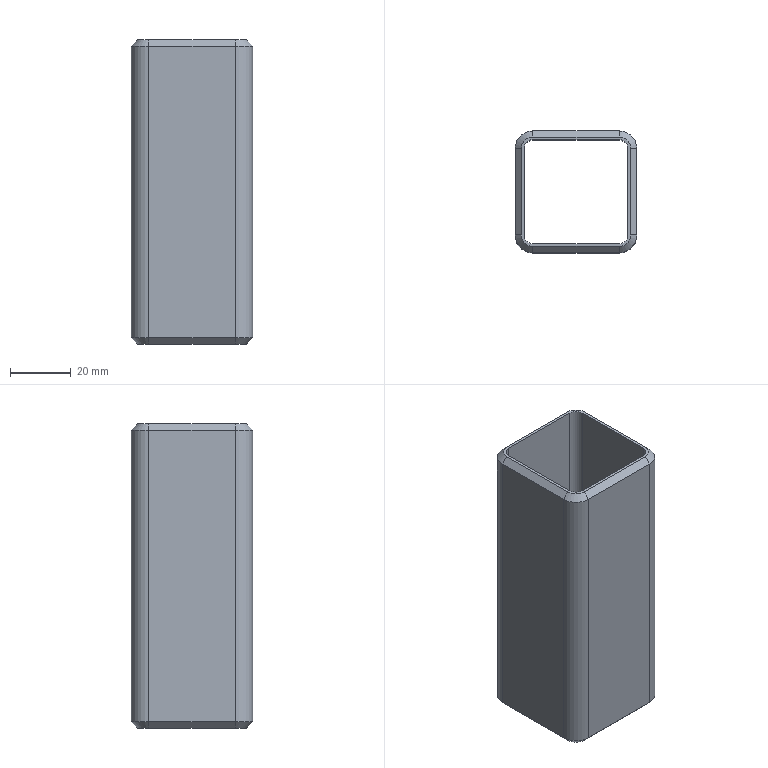Part | STEP file | IN-01-01-04-03 | 1 solid | 34 faces | box 40 x 40 x 100 mm | volume 40287 mm3 | plane 18 | cylinder 8 | cone 8 | commonest cylinder face diameters 5.8 x4 11.6 x4